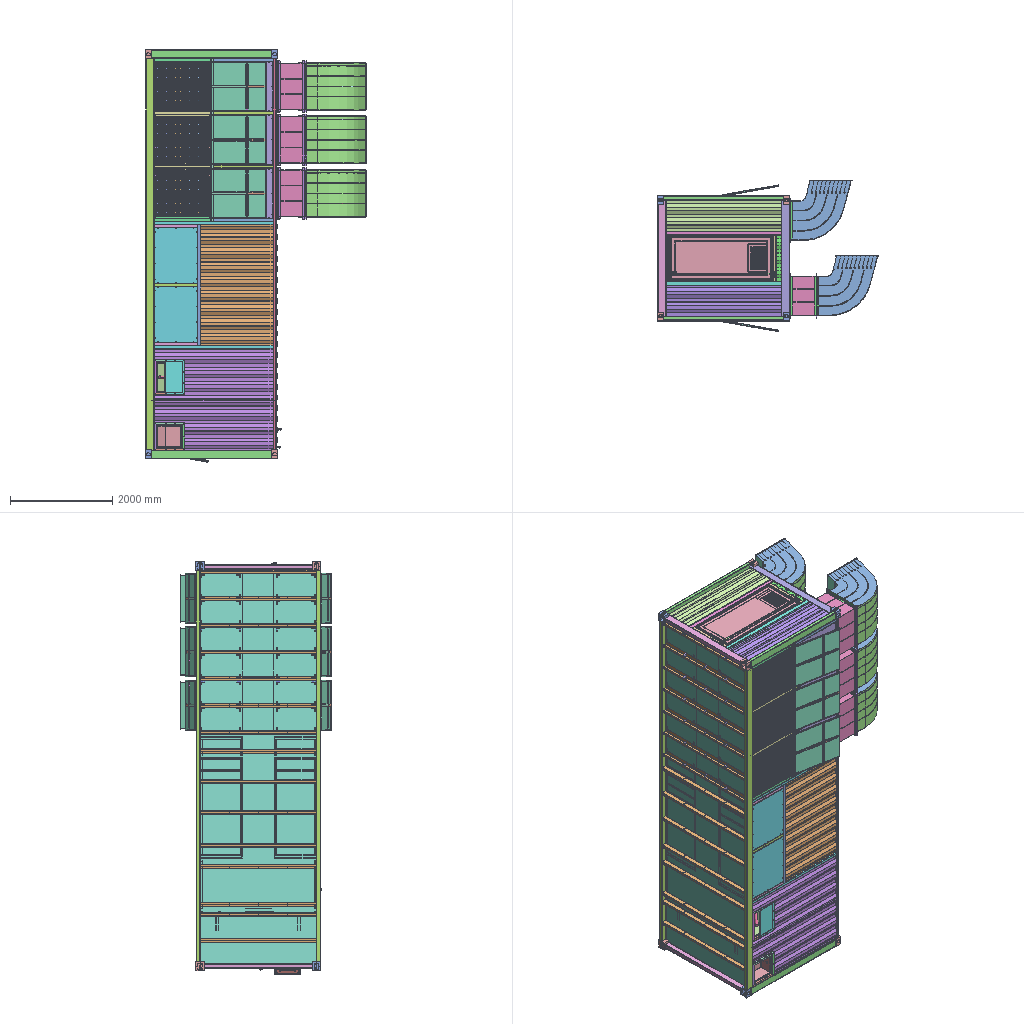Assembly | STEP file | 192 different items | 1741 placed | box 4327 x 2952 x 8065 mm
Parts list (item | name | quantity | parent item | size | volume):
1 | 750031822 | x2 | in 750038420 | 118 x 78 x 36 mm | 64893 mm3
2 | 750031823 | x2 | in 750038420 | 118 x 78 x 36 mm | 64892 mm3
3 | 750031837 | x4 | in 750038420 | 27.4 x 75 x 80 mm | 16937 mm3
4 | 750038121 | x15 | in 750038120 | 75 x 108 x 2272 mm | 1952553 mm3
5 | 750038122 | x45 | in 750038120 | 68 x 100 x 5 mm | 26375 mm3
6 | 750038132 | x3 | in 750038130 | 60 x 60 x 985 mm | 854437 mm3
7 | 750038133 | x6 | in 750038130, 750038135 | 12 x 12 x 60 mm | 2969 mm3
8 | 750038136 | x3 | in 750038135 | 60 x 60 x 985 mm | 854437 mm3
9 | 750038140 | x2 | in 750078100 | 43 x 80 x 2374 mm | 2431604 mm3
10 | 750038142 | x9 | in 750078100 | 1086 x 200 x 30 mm | 538093 mm3
11 | 750038150 | x4 | in 750078100 | 80 x 160 x 2355 mm | 5325530 mm3
12 | 750038152 | x4 | in 750078100 | 56 x 56 x 3 mm | 9385 mm3
13 | 750038153 | x5 | in 750078100 | 60 x 60 x 2327 mm | 2020637 mm3
14 | 750038156 | x2 | in 750078100 | 60 x 60 x 7644 mm | 6639051 mm3
15 | 750038157 | x4 | in 750078100 | 60 x 60 x 3195 mm | 2774956 mm3
16 | 750038160 | x8 | in 750078100 | 60 x 60 x 2312 mm | 2008044 mm3
17 | 750038161 | x2 | in 750078100 | 80 x 160 x 2272 mm | 4914158 mm3
18 | 750038163 | x2 | in 750078100 | 144 x 29 x 2114 mm | 1005017 mm3
19 | 750038164 | x2 | in 750078100 | 2360 x 36 x 1416 mm | 7069165 mm3
20 | 750038166 | x2 | in 750078100 | 884 x 1200 x 19.9 mm | 1728318 mm3
21 | 750038167 | x1 | in 750078100 | 4475 x 2356 x 19.9 mm | 17264106 mm3
22 | 750038168 | x1 | in 750078100 | 2428 x 2404 x 19.9 mm | 8825097 mm3
23 | 750038169 | x1 | in 750078100 | 1487 x 36 x 2327 mm | 7320463 mm3
24 | 750038170 | x10 | in 750078100 | 60 x 60 x 1160 mm | 1007496 mm3
25 | 750038172 | x8 | in 750078100 | 60 x 60 x 841 mm | 730435 mm3
26 | 750038173 | x1 | in 750078100 | 865 x 36 x 2253 mm | 3353740 mm3
27 | 750038175 | x1 | in 750078100 | 606 x 36 x 2253 mm | 2873440 mm3
28 | 750038176 | x2 | in 750078100 | 900 x 26 x 92.5 mm | 171034 mm3
29 | 750038178 | x1 | in 750078100 | 1997 x 36 x 2327 mm | 8230400 mm3
30 | 750038184 | x4 | in 750078100 | 154 x 27 x 1113 mm | 542434 mm3
31 | 750038185 | x4 | in 750078100 | 107 x 27 x 1113 mm | 364027 mm3
32 | 750038186 | x6 | in 750078100 | 47 x 35.779 x 981 mm | 158783 mm3
33 | 750038187 | x6 | in 750078100 | 47 x 35.779 x 981 mm | 158783 mm3
34 | 750038191 | x4 | in 750038190 | 84 x 27 x 1154 mm | 316306 mm3
35 | 750038193 | x4 | in 750038192 | 108 x 27.5 x 1154 mm | 435104 mm3
36 | 750038196 | x12 | in 750038195 | 24 x 15 x 981 mm | 68574 mm3
37 | 750038201 | x6 | in 750078100 | 154 x 140.678 x 33.357 mm | 8140 mm3
38 | 750038221 | x1 | in 750038220 | 500 x 148.5 x 150 mm | 178215 mm3
39 | 750038222 | x1 | in 750038220 | 250 x 150 x 1800 mm | 1443469 mm3
40 | 750038223 | x1 | in 750038220 | 496 x 30 x 153 mm | 126298 mm3
41 | 750038225 | x1 | in 750078000 | 255 x 21.5 x 1800 mm | 791285 mm3
42 | 750038227 | x2 | in 750078100 | 40 x 63 x 250 mm | 211142 mm3
43 | 750038228 | x4 | in 750078100 | 40 x 63 x 510 mm | 429975 mm3
44 | 750038229 | x3 | in 750078100 | 40 x 63 x 384 mm | 324314 mm3
45 | 750038230 | x5 | in 750078100 | 40 x 63 x 510 mm | 430729 mm3
46 | 750038231 | x6 | in 750078100 | 40 x 63 x 982 mm | 829365 mm3
47 | 750038232 | x1 | in 750078000 | 400 x 150 x 6614 mm | 7243143 mm3
48 | 750038235 | x1 | in 750078000 | 405 x 21.5 x 6614 mm | 4395351 mm3
49 | 750038236 | x1 | in 750078100 | 1044 x 507 x 10 mm | 5291709 mm3
50 | 750038237 | x2 | in 750078100 | 1074 x 507 x 10 mm | 5443022 mm3
51 | 750038241 | x10 | in 750038240 | 50 x 50 x 440 mm | 204554 mm3
52 | 750038242 | x20 | in 750038240 | 50 x 50 x 220 mm | 103128 mm3
53 | 750038243 | x10 | in 750038240 | 50 x 50 x 50 mm | 23258 mm3
54 | 750038244 | x10 | in 750038240 | 50 x 50 x 50 mm | 23258 mm3
55 | 750038245 | x20 | in 750078100 | 54 x 54 x 40 mm | 12946 mm3
56 | 750038251 | x2 | in 750038250 | 360 x 360 x 15 mm | 1468800 mm3
57 | 750038301 | x8 | in 750038300 | 30 x 60 x 1149 mm | 1566849 mm3
58 | 750038302 | x40 | in 750038300 | 15 x 5 x 50 mm | 3365 mm3
59 | 750038305 | x4 | in 110030150 | 30 x 60 x 1149 mm | 1861380 mm3
60 | 750038306 | x4 | in 110030150 | 30 x 60 x 1149 mm | 1360456 mm3
61 | 750038310 | x6 | in 110030150 | 1009 x 1149 x 10 mm | 10895411 mm3
62 | 750038315 | x6 | in 110030150 | 1009 x 1100 x 5 mm | 5535001 mm3
63 | 750038318 | x8 | in 110030150 | 845 x 1149 x 5 mm | 4854525 mm3
64 | 750038321 | x12 | in 750038320 | 25 x 30 x 1045 mm | 131869 mm3
65 | 750038326 | x16 | in 750038325 | 25 x 30 x 815 mm | 103040 mm3
66 | 750038331 | x12 | in 750038340_MODEL, 750038345_MODEL | 16.25 x 110 x 985 mm | 264288 mm3
67 | 750038332 | x84 | in 750038340_MODEL, 750038345_MODEL | 49 x 101 x 3 mm | 11694 mm3
68 | 750038333 | x12 | in 750038340_MODEL, 750038345_MODEL | 26 x 49 x 30 mm | 4154 mm3
69 | 750038334 | x12 | in 750038340_MODEL, 750038345_MODEL | 26 x 49 x 30 mm | 4154 mm3
70 | 750038351 | x7 | in 110030150 | 25 x 40 x 1214 mm | 1190455 mm3
71 | 750038353 | x1 | in 110030150 | 110.3 x 40.95 x 6 mm | 4017 mm3
72 | 750038381 | x6 | in 750038380 | 981 x 1150 x 23 mm | 1927525 mm3
73 | 750038384 | x6 | in 750078000 | 981 x 1150 x 3 mm | 275484 mm3
74 | 750038391 | x12 | in 750038390 | 43 x 33 x 1000 mm | 207432 mm3
75 | 750038392 | x12 | in 750038390 | 43 x 33 x 856 mm | 176921 mm3
76 | 750038395 | x1 | in 750078100 | 3095 x 610 x 3 mm | 5663850 mm3
77 | 750038400 | x2 | in 750078100 | 127 x 60 x 2253 mm | 1105749 mm3
78 | 750038401 | x2 | in 750078100 | 127 x 60 x 2253 mm | 1105749 mm3
79 | 750038402 | x4 | in 750078100 | 107 x 27 x 900 mm | 344520 mm3
80 | 750038404 | x3 | in 750038403 | 87 x 150 x 596 mm | 335193 mm3
81 | 750038405 | x4 | in 750038403 | 25 x 70 x 422 mm | 76342 mm3
82 | 750038406 | x16 | in 750038403, 750078410 | 41.359 x 45.634 x 422 mm | 39080 mm3
83 | 750038407 | x1 | in 750038403 | 600 x 600 x 51 mm | 373355 mm3
84 | 750038408 | x1 | in 750038403 | 600 x 600 x 44 mm | 824704 mm3
85 | 750038409 | x1 | in 750038403 | 87 x 120 x 596 mm | 299242 mm3
86 | 750038411 | x1 | in 750038410 | 896 x 2036 x 20 mm | 4018739 mm3
87 | 750038412 | x4 | in 750038410, 750078410 | 120 x 46.5 x 2028 mm | 584981 mm3
88 | 750038413 | x4 | in 750038410, 750078410 | 120 x 46.5 x 888 mm | 232487 mm3
89 | 750038414 | x1 | in 750038410 | 785 x 1925 x 1.5 mm | 2266688 mm3
90 | 750038419 | x2 | in 750038410, 750078410 | 881.505 x 20.12 x 2022 mm | 451078 mm3
91 | 750038421 | x2 | in 750038420 | 25.4 x 25.4 x 2024 mm | 1025576 mm3
92 | 750038430 | x8 | in 750078100 | 45 x 45 x 450 mm | 156442 mm3
93 | 750038433 | x1 | in 750078100 | 450 x 2327 x 100 mm | 3164012 mm3
94 | 750038446 | x2 | in 750038440 | 40 x 63 x 809.6 mm | 679679 mm3
95 | 750038447 | x48 | in 750038440 | 40 x 63 x 809.6 mm | 679680 mm3
96 | 750038448 | x2 | in 750038440 | 40 x 63 x 809.6 mm | 679680 mm3
97 | 750038449 | x4 | in 750038440 | 40 x 63 x 800 mm | 675654 mm3
98 | 750038452 | x8 | in 750038450 | 40 x 63 x 2262 mm | 1910749 mm3
99 | 750038453 | x8 | in 750038450 | 40 x 63 x 924 mm | 780380 mm3
100 | 750038454 | x12 | in 750038440, 750038450 | 40 x 63 x 2434 mm | 2055677 mm3
101 | 750038455 | x2 | in 750038450 | 40 x 63 x 924 mm | 777123 mm3
102 | 750038456 | x4 | in 750038450 | 40 x 63 x 924 mm | 773051 mm3
103 | 750038457 | x16 | in 750038440 | 40 x 63 x 810 mm | 684099 mm3
104 | 750038458 | x12 | in 750038450 | 40 x 63 x 924 mm | 779294 mm3
105 | 750038459 | x16 | in 750038440 | 40 x 63 x 2248 mm | 1898587 mm3
106 | 750038460 | x3 | in 110030150 | 700 x 80 x 6 mm | 330686 mm3
107 | 750038466 | x1 | in 750038465 | 70 x 50 x 696 mm | 223669 mm3
108 | 750038467 | x2 | in 750038465, 750038490 | 70 x 50 x 596 mm | 188466 mm3
109 | 750038468 | x1 | in 750038465 | 346.594 x 486 x 584 mm | 1359967 mm3
110 | 750038469 | x1 | in 110030150 | 497.894 x 1154 x 60 mm | 3628627 mm3
111 | 750038470 | x1 | in 750038465 | 70 x 50 x 696 mm | 223150 mm3
112 | 750038471 | x2 | in 750038465, 750038490 | 70 x 50 x 596 mm | 188466 mm3
113 | 750038472 | x1 | in 750078000 | 690 x 384 x 24 mm | 562921 mm3
114 | 750038473 | x1 | in 750078000 | 690 x 380 x 2 mm | 108343 mm3
115 | 750038481 | x4 | in 750038450 | 40 x 63 x 924 mm | 778209 mm3
116 | 750038491 | x1 | in 750038490 | 252 x 486 x 434 mm | 1098230 mm3
117 | 750038492 | x1 | in 750038490 | 70 x 50 x 546 mm | 171514 mm3
118 | 750038493 | x1 | in 750038490 | 70 x 50 x 546 mm | 171168 mm3
119 | 750038521 | x1 | in 750038520 | 514 x 514 x 20 mm | 656019 mm3
120 | 750038522 | x2 | in 750038520 | 120 x 21.5 x 508 mm | 88776 mm3
121 | 750038523 | x2 | in 750038520 | 120 x 21.5 x 508 mm | 88776 mm3
122 | 750038524 | x1 | in 750038520 | 405 x 405 x 1.5 mm | 246038 mm3
123 | 750038529 | x1 | in 750038520 | 501.538 x 20.12 x 501.538 mm | 180516 mm3
124 | 750038556 | x2 | in 750078100 | 1005 x 861 x 5 mm | 789021 mm3
125 | 750038561 | x2 | in 750038560 | 30 x 10 x 50 mm | 6694 mm3
126 | 750038562 | x2 | in 750038560 | 6 x 6 x 52 mm | 1243 mm3
127 | 750038563 | x2 | in 750038560 | 30 x 10 x 50 mm | 6670 mm3
128 | 750039230 | x2 | in 110030150 | 96 x 77 x 56 mm | 113749 mm3
129 | 750078111 | x2 | in 750078110 | 80 x 160 x 7672 mm | 17309604 mm3
130 | 750078112 | x2 | in 750078110 | 80 x 160 x 2272 mm | 4914158 mm3
131 | 750078135 | x1 | in 750078110 | 2272 x 7726 x 4 mm | 69829888 mm3
132 | 750078154 | x2 | in 750078100 | 60 x 60 x 2360 mm | 2049733 mm3
133 | 750078170 | x8 | in 750078100 | 60 x 60 x 1160 mm | 1007496 mm3
134 | 750078174 | x1 | in 750078100 | 347 x 36 x 2253 mm | 1650208 mm3
135 | 750078177 | x1 | in 750078100 | 606 x 36 x 2253 mm | 2873440 mm3
136 | 750078181 | x4 | in 750078180 | 52 x 20 x 889 mm | 95106 mm3
137 | 750078185 | x4 | in 750078184 | 52 x 20 x 1107 mm | 119219 mm3
138 | 750078188 | x6 | in 750078100 | 887 x 1018 x 3 mm | 516113 mm3
139 | 750078191 | x4 | in 750078190 | 84 x 27 x 850 mm | 232667 mm3
140 | 750078193 | x2 | in 750078192 | 108 x 27.5 x 850 mm | 319697 mm3
141 | 750078196 | x8 | in 750078195 | 24 x 15 x 1086 mm | 75901 mm3
142 | 750078200 | x6 | in 750078100 | 1025 x 915 x 6 mm | 3220443 mm3
143 | 750078212 | x6 | in 750078210_MODEL | 455 x 879 x 879 mm | 2524366 mm3
144 | 750078256 | x3 | in 750078255 | 40 x 420 x 985 mm | 948156 mm3
145 | 750078258 | x6 | in 750078255, 750078260 | 30 x 8 x 8 mm | 659.734 mm3
146 | 750078261 | x3 | in 750078260 | 40 x 420 x 985 mm | 948156 mm3
147 | 750078263 | x2 | in 750078262 | 25 x 30 x 985 mm | 118517 mm3
148 | 750078266 | x16 | in 750078265 | 25 x 30 x 704 mm | 84559 mm3
149 | 750078271 | x6 | in 750078270 | 979 x 758 x 17 mm | 1562109 mm3
150 | 750078273 | x2 | in 750078272 | 811 x 758 x 17 mm | 1299071 mm3
151 | 750078276 | x2 | in 750078275 | 40 x 420 x 817 mm | 786846 mm3
152 | 750078281 | x2 | in 750078280 | 25 x 30 x 817 mm | 98215 mm3
153 | 750078361 | x6 | in 750078360 | - | -
154 | 750078362 | x6 | in 750078360 | 974 x 21.5 x 55 mm | 128141 mm3
155 | 750078363 | x6 | in 750078360 | 699.5 x 21.5 x 55 mm | 93667 mm3
156 | 750078364 | x6 | in 750078360 | 366.5 x 21.5 x 55 mm | 47287 mm3
157 | 750078381 | x4 | in 750078380 | 1086 x 846 x 23 mm | 1590707 mm3
158 | 750078411 | x1 | in 750078410 | 896 x 2036 x 20 mm | 3760897 mm3
159 | 750078414 | x1 | in 750078410 | 785 x 1925 x 1.5 mm | 2064757 mm3
160 | 750078415 | x1 | in 750078410 | 70 x 46.5 x 539 mm | 119069 mm3
161 | 750078416 | x1 | in 750078410 | 70 x 46.5 x 374 mm | 85341 mm3
162 | 750078417 | x1 | in 750078410 | 70 x 46.5 x 374 mm | 85341 mm3
163 | 750078418 | x1 | in 750078410 | 422 x 305.5 x 1.5 mm | 45792 mm3
164 | 750078419 | x1 | in 750078410 | 275 x 82.5 x 25 mm | 170372 mm3
165 | 750078421 | x1 | in 750078420 | 471 x 366 x 20 mm | 448317 mm3
166 | 750078423 | x2 | in 750078410 | 60 x 25 x 20 mm | 30000 mm3
167 | 750078456 | x24 | in 750078455 | 50 x 40 x 1006 mm | 255301 mm3
168 | 750078457 | x24 | in 750078455 | 50 x 40 x 762 mm | 193524 mm3
169 | 750078461 | x6 | in 750078460 | 1184 x 1163 x 20 mm | 1210389 mm3
170 | 750078462 | x6 | in 750078460 | 1184 x 1163 x 20 mm | 1210382 mm3
171 | 750078463 | x6 | in 750078460 | 383.962 x 404.825 x 906 mm | 774801 mm3
172 | 750078464 | x6 | in 750078460 | 1203 x 1166 x 906 mm | 2297945 mm3
173 | 750078465 | x54 | in 750078460 | 250 x 25 x 892.6 mm | 322531 mm3
174 | 750078466 | x6 | in 750078460 | 19.319 x 9.272 x 903.6 mm | 29323 mm3
175 | 750078467 | x6 | in 750078460 | 19.629 x 30.176 x 903.6 mm | 47356 mm3
176 | 750078470 | x6 | in 750078450 | 938 x 833 x 3 mm | 434942 mm3
177 | 750078481 | x3 | in 750078480 | 906 x 762 x 500 mm | 2504428 mm3
178 | 921270125 | x4 | in 750078100, 750078110 | 118 x 162 x 178 mm | 2037441 mm3
179 | 921270126 | x4 | in 750078100, 750078110 | 118 x 162 x 178 mm | 2037103 mm3
180 | 921270223 | x2 | in 750078100 | 425 x 82.5 x 25 mm | 244003 mm3
181 | 921270336 | x108 | in 750038390 | 13 x 14.856 x 7.9 mm | 859.126 mm3
182 | 921271102 | x2 | in 110030150 | 10 x 11.547 x 5.2 mm | 337.323 mm3
183 | 921271103 | x1 | in 110030150 | 9.3 x 9.3 x 2 mm | 72.768 mm3
184 | 921271104 | x2 | in 110030150 | 12 x 12 x 1.6 mm | 126.217 mm3
185 | 921271505 | x68 | in 110030150, 750078000, 750078100 | 40 x 30 x 25 mm | 3358 mm3
186 | 921272110 | x12 | in 921272100 | 520 x 243 x 450 mm | 26860922 mm3
187 | 921272131 | x3 | in 921272130 | 310 x 180 x 300 mm | 11781247 mm3
188 | 921272141 | x2 | in 921272140 | 287 x 190 x 252 mm | 8017788 mm3
189 | 921272175 | x6 | in 110030150 | 200 x 200 x 265 mm | 3161533 mm3
190 | 921281610 | x60 | in 750038240 | 13 x 15.011 x 30.3 mm | 2021 mm3
191 | 921281612 | x60 | in 750038240 | 13 x 14.856 x 7.9 mm | 859.126 mm3
192 | 921292560 | x327 | in 750038190, 750038192, 750038195, 750038320, 750038325, 750038340_MODEL, 750038345_MODEL, 750038465, 750038490, 750078180, 750078184, 750078192, 750078255, 750078260, 750078262, 750078265, 750078275, 750078280 | 12.5 x 6.38 x 12.5 mm | 499.816 mm3